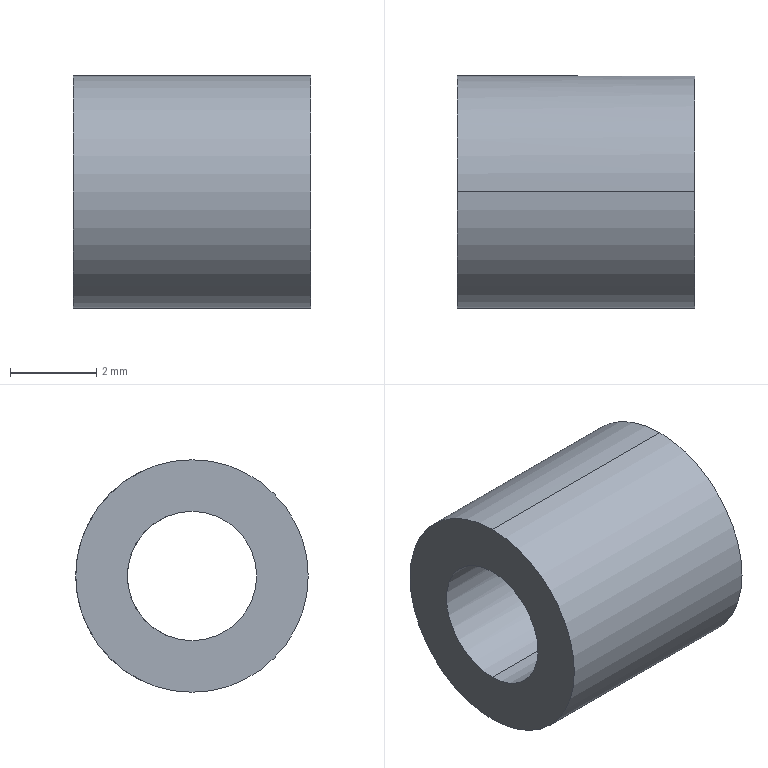Part | STEP file | RJ-HMS7-01_X2_58F34F5394A391D_1 | 1 solid | 6 faces | box 5.5 x 5.39 x 5.39 mm | volume 86.619 mm3 | cylinder 4 | plane 2 | commonest cylinder face diameters 3 x2 5.39 x2
STEP:
#1=CARTESIAN_POINT('',(0.,0.,0.));
#2=DIRECTION('',(0.,0.,1.));
#3=DIRECTION('',(1.,0.,0.));
#4=AXIS2_PLACEMENT_3D('',#1,#2,#3);
#5=CARTESIAN_POINT('',(762.8,4073.828,1374.941));
#6=VERTEX_POINT('',#5);
#7=CARTESIAN_POINT('',(762.8,4076.523,1372.246));
#8=VERTEX_POINT('',#7);
#9=CARTESIAN_POINT('',(762.8,4073.828,1372.246));
#10=DIRECTION('',(-1.,0.,0.));
#11=DIRECTION('',(0.,0.,1.));
#12=AXIS2_PLACEMENT_3D('',#9,#10,#11);
#13=CIRCLE('',#12,2.695);
#14=CARTESIAN_POINT('',(762.8,4073.828,1372.246));
#15=DIRECTION('',(1.,0.,0.));
#16=DIRECTION('',(0.,0.,-1.));
#17=AXIS2_PLACEMENT_3D('',#14,#15,#16);
#18=CYLINDRICAL_SURFACE('',#17,2.695);
#19=CARTESIAN_POINT('',(3.142,0.));
#20=DIRECTION('',(-1.,0.));
#21=VECTOR('',#20,1.);
#22=LINE('',#19,#21);
#23=(GEOMETRIC_REPRESENTATION_CONTEXT(2)PARAMETRIC_REPRESENTATION_CONTEXT()REPRESENTATION_CONTEXT('',''));
#24=DEFINITIONAL_REPRESENTATION('',(#22),#23);
#25=PCURVE('',#18,#24);
#26=CARTESIAN_POINT('',(762.8,4073.828,1372.246));
#27=DIRECTION('',(-1.,0.,0.));
#28=DIRECTION('',(0.,0.,1.));
#29=AXIS2_PLACEMENT_3D('',#26,#27,#28);
#30=PLANE('',#29);
#31=CARTESIAN_POINT('',(0.,0.));
#32=DIRECTION('',(1.,0.));
#33=AXIS2_PLACEMENT_2D('',#31,#32);
#34=CIRCLE('',#33,2.695);
#35=(GEOMETRIC_REPRESENTATION_CONTEXT(2)PARAMETRIC_REPRESENTATION_CONTEXT()REPRESENTATION_CONTEXT('',''));
#36=DEFINITIONAL_REPRESENTATION('',(#34),#35);
#37=PCURVE('',#30,#36);
#38=SURFACE_CURVE('',#13,(#25,#37),.PCURVE_S1.);
#39=EDGE_CURVE('',#6,#8,#38,.T.);
#40=ORIENTED_EDGE('',*,*,#39,.F.);
#41=CARTESIAN_POINT('',(768.3,4073.828,1374.941));
#42=VERTEX_POINT('',#41);
#43=CARTESIAN_POINT('',(762.8,4073.828,1374.941));
#44=DIRECTION('',(1.,0.,0.));
#45=VECTOR('',#44,1.);
#46=LINE('',#43,#45);
#47=CARTESIAN_POINT('',(3.142,0.));
#48=DIRECTION('',(0.,1.));
#49=VECTOR('',#48,1.);
#50=LINE('',#47,#49);
#51=(GEOMETRIC_REPRESENTATION_CONTEXT(2)PARAMETRIC_REPRESENTATION_CONTEXT()REPRESENTATION_CONTEXT('',''));
#52=DEFINITIONAL_REPRESENTATION('',(#50),#51);
#53=PCURVE('',#18,#52);
#54=CARTESIAN_POINT('',(762.8,4073.828,1372.246));
#55=DIRECTION('',(1.,0.,0.));
#56=DIRECTION('',(0.,0.,-1.));
#57=AXIS2_PLACEMENT_3D('',#54,#55,#56);
#58=CYLINDRICAL_SURFACE('',#57,2.695);
#59=CARTESIAN_POINT('',(3.142,0.));
#60=DIRECTION('',(0.,1.));
#61=VECTOR('',#60,1.);
#62=LINE('',#59,#61);
#63=(GEOMETRIC_REPRESENTATION_CONTEXT(2)PARAMETRIC_REPRESENTATION_CONTEXT()REPRESENTATION_CONTEXT('',''));
#64=DEFINITIONAL_REPRESENTATION('',(#62),#63);
#65=PCURVE('',#58,#64);
#66=SURFACE_CURVE('',#46,(#53,#65),.PCURVE_S1.);
#67=EDGE_CURVE('',#6,#42,#66,.T.);
#68=ORIENTED_EDGE('',*,*,#67,.T.);
#69=CARTESIAN_POINT('',(768.3,4073.828,1369.551));
#70=VERTEX_POINT('',#69);
#71=CARTESIAN_POINT('',(768.3,4073.828,1372.246));
#72=DIRECTION('',(1.,0.,0.));
#73=DIRECTION('',(0.,0.,-1.));
#74=AXIS2_PLACEMENT_3D('',#71,#72,#73);
#75=CIRCLE('',#74,2.695);
#76=CARTESIAN_POINT('',(0.,5.5));
#77=DIRECTION('',(1.,0.));
#78=VECTOR('',#77,1.);
#79=LINE('',#76,#78);
#80=(GEOMETRIC_REPRESENTATION_CONTEXT(2)PARAMETRIC_REPRESENTATION_CONTEXT()REPRESENTATION_CONTEXT('',''));
#81=DEFINITIONAL_REPRESENTATION('',(#79),#80);
#82=PCURVE('',#18,#81);
#83=CARTESIAN_POINT('',(768.3,4073.828,1372.246));
#84=DIRECTION('',(-1.,0.,0.));
#85=DIRECTION('',(0.,0.,1.));
#86=AXIS2_PLACEMENT_3D('',#83,#84,#85);
#87=PLANE('',#86);
#88=CARTESIAN_POINT('',(-2.695,0.));
#89=CARTESIAN_POINT('',(-2.695,4.668));
#90=CARTESIAN_POINT('',(1.347,2.334));
#91=CARTESIAN_POINT('',(5.39,0.));
#92=CARTESIAN_POINT('',(1.347,-2.334));
#93=CARTESIAN_POINT('',(-2.695,-4.668));
#94=CARTESIAN_POINT('',(-2.695,0.));
#95=(BOUNDED_CURVE()B_SPLINE_CURVE(2,(#88,#89,#90,#91,#92,#93,#94),.UNSPECIFIED.,.T.,.F.)B_SPLINE_CURVE_WITH_KNOTS((1,2,2,2,2,1),(-2.094,0.,2.094,4.189,6.283,8.378),.UNSPECIFIED.)CURVE()GEOMETRIC_REPRESENTATION_ITEM()RATIONAL_B_SPLINE_CURVE((1.,0.5,1.,0.5,1.,0.5,1.))REPRESENTATION_ITEM(''));
#96=(GEOMETRIC_REPRESENTATION_CONTEXT(2)PARAMETRIC_REPRESENTATION_CONTEXT()REPRESENTATION_CONTEXT('',''));
#97=DEFINITIONAL_REPRESENTATION('',(#95),#96);
#98=PCURVE('',#87,#97);
#99=SURFACE_CURVE('',#75,(#82,#98),.PCURVE_S1.);
#100=EDGE_CURVE('',#70,#42,#99,.T.);
#101=ORIENTED_EDGE('',*,*,#100,.F.);
#102=CARTESIAN_POINT('',(762.8,4073.828,1369.551));
#103=VERTEX_POINT('',#102);
#104=CARTESIAN_POINT('',(762.8,4073.828,1369.551));
#105=DIRECTION('',(1.,0.,0.));
#106=VECTOR('',#105,1.);
#107=LINE('',#104,#106);
#108=CARTESIAN_POINT('',(0.,0.));
#109=DIRECTION('',(0.,1.));
#110=VECTOR('',#109,1.);
#111=LINE('',#108,#110);
#112=(GEOMETRIC_REPRESENTATION_CONTEXT(2)PARAMETRIC_REPRESENTATION_CONTEXT()REPRESENTATION_CONTEXT('',''));
#113=DEFINITIONAL_REPRESENTATION('',(#111),#112);
#114=PCURVE('',#18,#113);
#115=CARTESIAN_POINT('',(6.283,0.));
#116=DIRECTION('',(0.,1.));
#117=VECTOR('',#116,1.);
#118=LINE('',#115,#117);
#119=(GEOMETRIC_REPRESENTATION_CONTEXT(2)PARAMETRIC_REPRESENTATION_CONTEXT()REPRESENTATION_CONTEXT('',''));
#120=DEFINITIONAL_REPRESENTATION('',(#118),#119);
#121=PCURVE('',#58,#120);
#122=SURFACE_CURVE('',#107,(#114,#121),.PCURVE_S1.);
#123=EDGE_CURVE('',#103,#70,#122,.T.);
#124=ORIENTED_EDGE('',*,*,#123,.F.);
#125=CARTESIAN_POINT('',(762.8,4073.828,1372.246));
#126=DIRECTION('',(-1.,0.,0.));
#127=DIRECTION('',(0.,1.,0.));
#128=AXIS2_PLACEMENT_3D('',#125,#126,#127);
#129=CIRCLE('',#128,2.695);
#130=CARTESIAN_POINT('',(1.571,0.));
#131=DIRECTION('',(-1.,0.));
#132=VECTOR('',#131,1.);
#133=LINE('',#130,#132);
#134=(GEOMETRIC_REPRESENTATION_CONTEXT(2)PARAMETRIC_REPRESENTATION_CONTEXT()REPRESENTATION_CONTEXT('',''));
#135=DEFINITIONAL_REPRESENTATION('',(#133),#134);
#136=PCURVE('',#18,#135);
#137=CARTESIAN_POINT('',(0.,0.));
#138=DIRECTION('',(0.,1.));
#139=AXIS2_PLACEMENT_2D('',#137,#138);
#140=CIRCLE('',#139,2.695);
#141=(GEOMETRIC_REPRESENTATION_CONTEXT(2)PARAMETRIC_REPRESENTATION_CONTEXT()REPRESENTATION_CONTEXT('',''));
#142=DEFINITIONAL_REPRESENTATION('',(#140),#141);
#143=PCURVE('',#30,#142);
#144=SURFACE_CURVE('',#129,(#136,#143),.PCURVE_S1.);
#145=EDGE_CURVE('',#8,#103,#144,.T.);
#146=ORIENTED_EDGE('',*,*,#145,.F.);
#147=EDGE_LOOP('',(#40,#68,#101,#124,#146));
#148=FACE_BOUND('',#147,.T.);
#149=ADVANCED_FACE('',(#148),#18,.T.);
#150=CARTESIAN_POINT('',(762.8,4071.133,1372.246));
#151=VERTEX_POINT('',#150);
#152=CARTESIAN_POINT('',(762.8,4073.828,1372.246));
#153=DIRECTION('',(-1.,0.,0.));
#154=DIRECTION('',(0.,-1.,0.));
#155=AXIS2_PLACEMENT_3D('',#152,#153,#154);
#156=CIRCLE('',#155,2.695);
#157=CARTESIAN_POINT('',(0.,0.));
#158=DIRECTION('',(0.,-1.));
#159=AXIS2_PLACEMENT_2D('',#157,#158);
#160=CIRCLE('',#159,2.695);
#161=(GEOMETRIC_REPRESENTATION_CONTEXT(2)PARAMETRIC_REPRESENTATION_CONTEXT()REPRESENTATION_CONTEXT('',''));
#162=DEFINITIONAL_REPRESENTATION('',(#160),#161);
#163=PCURVE('',#30,#162);
#164=CARTESIAN_POINT('',(4.712,0.));
#165=DIRECTION('',(-1.,0.));
#166=VECTOR('',#165,1.);
#167=LINE('',#164,#166);
#168=(GEOMETRIC_REPRESENTATION_CONTEXT(2)PARAMETRIC_REPRESENTATION_CONTEXT()REPRESENTATION_CONTEXT('',''));
#169=DEFINITIONAL_REPRESENTATION('',(#167),#168);
#170=PCURVE('',#58,#169);
#171=SURFACE_CURVE('',#156,(#163,#170),.PCURVE_S1.);
#172=EDGE_CURVE('',#151,#6,#171,.T.);
#173=ORIENTED_EDGE('',*,*,#172,.F.);
#174=CARTESIAN_POINT('',(762.8,4073.828,1372.246));
#175=DIRECTION('',(-1.,0.,0.));
#176=DIRECTION('',(0.,0.,-1.));
#177=AXIS2_PLACEMENT_3D('',#174,#175,#176);
#178=CIRCLE('',#177,2.695);
#179=CARTESIAN_POINT('',(0.,0.));
#180=DIRECTION('',(-1.,0.));
#181=AXIS2_PLACEMENT_2D('',#179,#180);
#182=CIRCLE('',#181,2.695);
#183=(GEOMETRIC_REPRESENTATION_CONTEXT(2)PARAMETRIC_REPRESENTATION_CONTEXT()REPRESENTATION_CONTEXT('',''));
#184=DEFINITIONAL_REPRESENTATION('',(#182),#183);
#185=PCURVE('',#30,#184);
#186=CARTESIAN_POINT('',(6.283,0.));
#187=DIRECTION('',(-1.,0.));
#188=VECTOR('',#187,1.);
#189=LINE('',#186,#188);
#190=(GEOMETRIC_REPRESENTATION_CONTEXT(2)PARAMETRIC_REPRESENTATION_CONTEXT()REPRESENTATION_CONTEXT('',''));
#191=DEFINITIONAL_REPRESENTATION('',(#189),#190);
#192=PCURVE('',#58,#191);
#193=SURFACE_CURVE('',#178,(#185,#192),.PCURVE_S1.);
#194=EDGE_CURVE('',#103,#151,#193,.T.);
#195=ORIENTED_EDGE('',*,*,#194,.F.);
#196=ORIENTED_EDGE('',*,*,#145,.F.);
#197=ORIENTED_EDGE('',*,*,#39,.F.);
#198=EDGE_LOOP('',(#173,#195,#196,#197));
#199=FACE_BOUND('',#198,.F.);
#200=CARTESIAN_POINT('',(762.8,4072.328,1372.246));
#201=VERTEX_POINT('',#200);
#202=CARTESIAN_POINT('',(762.8,4073.828,1370.746));
#203=VERTEX_POINT('',#202);
#204=CARTESIAN_POINT('',(762.8,4073.828,1372.246));
#205=DIRECTION('',(1.,0.,0.));
#206=DIRECTION('',(0.,-1.,0.));
#207=AXIS2_PLACEMENT_3D('',#204,#205,#206);
#208=CIRCLE('',#207,1.5);
#209=CARTESIAN_POINT('',(0.,-1.5));
#210=CARTESIAN_POINT('',(-2.598,-1.5));
#211=CARTESIAN_POINT('',(-1.299,0.75));
#212=CARTESIAN_POINT('',(0.,3.));
#213=CARTESIAN_POINT('',(1.299,0.75));
#214=CARTESIAN_POINT('',(2.598,-1.5));
#215=CARTESIAN_POINT('',(0.,-1.5));
#216=(BOUNDED_CURVE()B_SPLINE_CURVE(2,(#209,#210,#211,#212,#213,#214,#215),.UNSPECIFIED.,.T.,.F.)B_SPLINE_CURVE_WITH_KNOTS((1,2,2,2,2,1),(-2.094,0.,2.094,4.189,6.283,8.378),.UNSPECIFIED.)CURVE()GEOMETRIC_REPRESENTATION_ITEM()RATIONAL_B_SPLINE_CURVE((1.,0.5,1.,0.5,1.,0.5,1.))REPRESENTATION_ITEM(''));
#217=(GEOMETRIC_REPRESENTATION_CONTEXT(2)PARAMETRIC_REPRESENTATION_CONTEXT()REPRESENTATION_CONTEXT('',''));
#218=DEFINITIONAL_REPRESENTATION('',(#216),#217);
#219=PCURVE('',#30,#218);
#220=CARTESIAN_POINT('',(762.8,4073.828,1372.246));
#221=DIRECTION('',(1.,0.,0.));
#222=DIRECTION('',(0.,0.,-1.));
#223=AXIS2_PLACEMENT_3D('',#220,#221,#222);
#224=CYLINDRICAL_SURFACE('',#223,1.5);
#225=CARTESIAN_POINT('',(4.712,0.));
#226=DIRECTION('',(1.,0.));
#227=VECTOR('',#226,1.);
#228=LINE('',#225,#227);
#229=(GEOMETRIC_REPRESENTATION_CONTEXT(2)PARAMETRIC_REPRESENTATION_CONTEXT()REPRESENTATION_CONTEXT('',''));
#230=DEFINITIONAL_REPRESENTATION('',(#228),#229);
#231=PCURVE('',#224,#230);
#232=SURFACE_CURVE('',#208,(#219,#231),.PCURVE_S1.);
#233=EDGE_CURVE('',#201,#203,#232,.T.);
#234=ORIENTED_EDGE('',*,*,#233,.F.);
#235=CARTESIAN_POINT('',(762.8,4073.828,1373.746));
#236=VERTEX_POINT('',#235);
#237=CARTESIAN_POINT('',(762.8,4073.828,1372.246));
#238=DIRECTION('',(1.,0.,0.));
#239=DIRECTION('',(0.,0.,1.));
#240=AXIS2_PLACEMENT_3D('',#237,#238,#239);
#241=CIRCLE('',#240,1.5);
#242=CARTESIAN_POINT('',(1.5,0.));
#243=CARTESIAN_POINT('',(1.5,-2.598));
#244=CARTESIAN_POINT('',(-0.75,-1.299));
#245=CARTESIAN_POINT('',(-3.,0.));
#246=CARTESIAN_POINT('',(-0.75,1.299));
#247=CARTESIAN_POINT('',(1.5,2.598));
#248=CARTESIAN_POINT('',(1.5,0.));
#249=(BOUNDED_CURVE()B_SPLINE_CURVE(2,(#242,#243,#244,#245,#246,#247,#248),.UNSPECIFIED.,.T.,.F.)B_SPLINE_CURVE_WITH_KNOTS((1,2,2,2,2,1),(-2.094,0.,2.094,4.189,6.283,8.378),.UNSPECIFIED.)CURVE()GEOMETRIC_REPRESENTATION_ITEM()RATIONAL_B_SPLINE_CURVE((1.,0.5,1.,0.5,1.,0.5,1.))REPRESENTATION_ITEM(''));
#250=(GEOMETRIC_REPRESENTATION_CONTEXT(2)PARAMETRIC_REPRESENTATION_CONTEXT()REPRESENTATION_CONTEXT('',''));
#251=DEFINITIONAL_REPRESENTATION('',(#249),#250);
#252=PCURVE('',#30,#251);
#253=CARTESIAN_POINT('',(3.142,0.));
#254=DIRECTION('',(1.,0.));
#255=VECTOR('',#254,1.);
#256=LINE('',#253,#255);
#257=(GEOMETRIC_REPRESENTATION_CONTEXT(2)PARAMETRIC_REPRESENTATION_CONTEXT()REPRESENTATION_CONTEXT('',''));
#258=DEFINITIONAL_REPRESENTATION('',(#256),#257);
#259=PCURVE('',#224,#258);
#260=SURFACE_CURVE('',#241,(#252,#259),.PCURVE_S1.);
#261=EDGE_CURVE('',#236,#201,#260,.T.);
#262=ORIENTED_EDGE('',*,*,#261,.F.);
#263=CARTESIAN_POINT('',(762.8,4073.828,1372.246));
#264=DIRECTION('',(1.,0.,0.));
#265=DIRECTION('',(0.,0.,-1.));
#266=AXIS2_PLACEMENT_3D('',#263,#264,#265);
#267=CIRCLE('',#266,1.5);
#268=CARTESIAN_POINT('',(-1.5,0.));
#269=CARTESIAN_POINT('',(-1.5,2.598));
#270=CARTESIAN_POINT('',(0.75,1.299));
#271=CARTESIAN_POINT('',(3.,0.));
#272=CARTESIAN_POINT('',(0.75,-1.299));
#273=CARTESIAN_POINT('',(-1.5,-2.598));
#274=CARTESIAN_POINT('',(-1.5,0.));
#275=(BOUNDED_CURVE()B_SPLINE_CURVE(2,(#268,#269,#270,#271,#272,#273,#274),.UNSPECIFIED.,.T.,.F.)B_SPLINE_CURVE_WITH_KNOTS((1,2,2,2,2,1),(-2.094,0.,2.094,4.189,6.283,8.378),.UNSPECIFIED.)CURVE()GEOMETRIC_REPRESENTATION_ITEM()RATIONAL_B_SPLINE_CURVE((1.,0.5,1.,0.5,1.,0.5,1.))REPRESENTATION_ITEM(''));
#276=(GEOMETRIC_REPRESENTATION_CONTEXT(2)PARAMETRIC_REPRESENTATION_CONTEXT()REPRESENTATION_CONTEXT('',''));
#277=DEFINITIONAL_REPRESENTATION('',(#275),#276);
#278=PCURVE('',#30,#277);
#279=CARTESIAN_POINT('',(762.8,4073.828,1372.246));
#280=DIRECTION('',(1.,0.,0.));
#281=DIRECTION('',(0.,0.,-1.));
#282=AXIS2_PLACEMENT_3D('',#279,#280,#281);
#283=CYLINDRICAL_SURFACE('',#282,1.5);
#284=CARTESIAN_POINT('',(0.,0.));
#285=DIRECTION('',(1.,0.));
#286=VECTOR('',#285,1.);
#287=LINE('',#284,#286);
#288=(GEOMETRIC_REPRESENTATION_CONTEXT(2)PARAMETRIC_REPRESENTATION_CONTEXT()REPRESENTATION_CONTEXT('',''));
#289=DEFINITIONAL_REPRESENTATION('',(#287),#288);
#290=PCURVE('',#283,#289);
#291=SURFACE_CURVE('',#267,(#278,#290),.PCURVE_S1.);
#292=EDGE_CURVE('',#203,#236,#291,.T.);
#293=ORIENTED_EDGE('',*,*,#292,.F.);
#294=EDGE_LOOP('',(#234,#262,#293));
#295=FACE_BOUND('',#294,.F.);
#296=ADVANCED_FACE('',(#199,#295),#30,.T.);
#297=ORIENTED_EDGE('',*,*,#123,.T.);
#298=CARTESIAN_POINT('',(768.3,4071.133,1372.246));
#299=VERTEX_POINT('',#298);
#300=CARTESIAN_POINT('',(768.3,4073.828,1372.246));
#301=DIRECTION('',(1.,0.,0.));
#302=DIRECTION('',(0.,-1.,0.));
#303=AXIS2_PLACEMENT_3D('',#300,#301,#302);
#304=CIRCLE('',#303,2.695);
#305=CARTESIAN_POINT('',(4.712,5.5));
#306=DIRECTION('',(1.,0.));
#307=VECTOR('',#306,1.);
#308=LINE('',#305,#307);
#309=(GEOMETRIC_REPRESENTATION_CONTEXT(2)PARAMETRIC_REPRESENTATION_CONTEXT()REPRESENTATION_CONTEXT('',''));
#310=DEFINITIONAL_REPRESENTATION('',(#308),#309);
#311=PCURVE('',#58,#310);
#312=CARTESIAN_POINT('',(0.,-2.695));
#313=CARTESIAN_POINT('',(-4.668,-2.695));
#314=CARTESIAN_POINT('',(-2.334,1.347));
#315=CARTESIAN_POINT('',(0.,5.39));
#316=CARTESIAN_POINT('',(2.334,1.347));
#317=CARTESIAN_POINT('',(4.668,-2.695));
#318=CARTESIAN_POINT('',(0.,-2.695));
#319=(BOUNDED_CURVE()B_SPLINE_CURVE(2,(#312,#313,#314,#315,#316,#317,#318),.UNSPECIFIED.,.T.,.F.)B_SPLINE_CURVE_WITH_KNOTS((1,2,2,2,2,1),(-2.094,0.,2.094,4.189,6.283,8.378),.UNSPECIFIED.)CURVE()GEOMETRIC_REPRESENTATION_ITEM()RATIONAL_B_SPLINE_CURVE((1.,0.5,1.,0.5,1.,0.5,1.))REPRESENTATION_ITEM(''));
#320=(GEOMETRIC_REPRESENTATION_CONTEXT(2)PARAMETRIC_REPRESENTATION_CONTEXT()REPRESENTATION_CONTEXT('',''));
#321=DEFINITIONAL_REPRESENTATION('',(#319),#320);
#322=PCURVE('',#87,#321);
#323=SURFACE_CURVE('',#304,(#311,#322),.PCURVE_S1.);
#324=EDGE_CURVE('',#299,#70,#323,.T.);
#325=ORIENTED_EDGE('',*,*,#324,.F.);
#326=CARTESIAN_POINT('',(768.3,4073.828,1372.246));
#327=DIRECTION('',(1.,0.,0.));
#328=DIRECTION('',(0.,0.,1.));
#329=AXIS2_PLACEMENT_3D('',#326,#327,#328);
#330=CIRCLE('',#329,2.695);
#331=CARTESIAN_POINT('',(3.142,5.5));
#332=DIRECTION('',(1.,0.));
#333=VECTOR('',#332,1.);
#334=LINE('',#331,#333);
#335=(GEOMETRIC_REPRESENTATION_CONTEXT(2)PARAMETRIC_REPRESENTATION_CONTEXT()REPRESENTATION_CONTEXT('',''));
#336=DEFINITIONAL_REPRESENTATION('',(#334),#335);
#337=PCURVE('',#58,#336);
#338=CARTESIAN_POINT('',(2.695,0.));
#339=CARTESIAN_POINT('',(2.695,-4.668));
#340=CARTESIAN_POINT('',(-1.347,-2.334));
#341=CARTESIAN_POINT('',(-5.39,0.));
#342=CARTESIAN_POINT('',(-1.347,2.334));
#343=CARTESIAN_POINT('',(2.695,4.668));
#344=CARTESIAN_POINT('',(2.695,0.));
#345=(BOUNDED_CURVE()B_SPLINE_CURVE(2,(#338,#339,#340,#341,#342,#343,#344),.UNSPECIFIED.,.T.,.F.)B_SPLINE_CURVE_WITH_KNOTS((1,2,2,2,2,1),(-2.094,0.,2.094,4.189,6.283,8.378),.UNSPECIFIED.)CURVE()GEOMETRIC_REPRESENTATION_ITEM()RATIONAL_B_SPLINE_CURVE((1.,0.5,1.,0.5,1.,0.5,1.))REPRESENTATION_ITEM(''));
#346=(GEOMETRIC_REPRESENTATION_CONTEXT(2)PARAMETRIC_REPRESENTATION_CONTEXT()REPRESENTATION_CONTEXT('',''));
#347=DEFINITIONAL_REPRESENTATION('',(#345),#346);
#348=PCURVE('',#87,#347);
#349=SURFACE_CURVE('',#330,(#337,#348),.PCURVE_S1.);
#350=EDGE_CURVE('',#42,#299,#349,.T.);
#351=ORIENTED_EDGE('',*,*,#350,.F.);
#352=ORIENTED_EDGE('',*,*,#67,.F.);
#353=ORIENTED_EDGE('',*,*,#172,.F.);
#354=ORIENTED_EDGE('',*,*,#194,.F.);
#355=EDGE_LOOP('',(#297,#325,#351,#352,#353,#354));
#356=FACE_BOUND('',#355,.T.);
#357=ADVANCED_FACE('',(#356),#58,.T.);
#358=ORIENTED_EDGE('',*,*,#324,.F.);
#359=ORIENTED_EDGE('',*,*,#350,.F.);
#360=ORIENTED_EDGE('',*,*,#100,.F.);
#361=EDGE_LOOP('',(#358,#359,#360));
#362=FACE_BOUND('',#361,.F.);
#363=CARTESIAN_POINT('',(768.3,4072.328,1372.246));
#364=VERTEX_POINT('',#363);
#365=CARTESIAN_POINT('',(768.3,4073.828,1373.746));
#366=VERTEX_POINT('',#365);
#367=CARTESIAN_POINT('',(768.3,4073.828,1372.246));
#368=DIRECTION('',(-1.,0.,0.));
#369=DIRECTION('',(0.,-1.,0.));
#370=AXIS2_PLACEMENT_3D('',#367,#368,#369);
#371=CIRCLE('',#370,1.5);
#372=CARTESIAN_POINT('',(0.,0.));
#373=DIRECTION('',(0.,-1.));
#374=AXIS2_PLACEMENT_2D('',#372,#373);
#375=CIRCLE('',#374,1.5);
#376=(GEOMETRIC_REPRESENTATION_CONTEXT(2)PARAMETRIC_REPRESENTATION_CONTEXT()REPRESENTATION_CONTEXT('',''));
#377=DEFINITIONAL_REPRESENTATION('',(#375),#376);
#378=PCURVE('',#87,#377);
#379=CARTESIAN_POINT('',(4.712,5.5));
#380=DIRECTION('',(-1.,0.));
#381=VECTOR('',#380,1.);
#382=LINE('',#379,#381);
#383=(GEOMETRIC_REPRESENTATION_CONTEXT(2)PARAMETRIC_REPRESENTATION_CONTEXT()REPRESENTATION_CONTEXT('',''));
#384=DEFINITIONAL_REPRESENTATION('',(#382),#383);
#385=PCURVE('',#224,#384);
#386=SURFACE_CURVE('',#371,(#378,#385),.PCURVE_S1.);
#387=EDGE_CURVE('',#364,#366,#386,.T.);
#388=ORIENTED_EDGE('',*,*,#387,.F.);
#389=CARTESIAN_POINT('',(768.3,4073.828,1370.746));
#390=VERTEX_POINT('',#389);
#391=CARTESIAN_POINT('',(768.3,4073.828,1372.246));
#392=DIRECTION('',(-1.,0.,0.));
#393=DIRECTION('',(0.,0.,-1.));
#394=AXIS2_PLACEMENT_3D('',#391,#392,#393);
#395=CIRCLE('',#394,1.5);
#396=CARTESIAN_POINT('',(0.,0.));
#397=DIRECTION('',(-1.,0.));
#398=AXIS2_PLACEMENT_2D('',#396,#397);
#399=CIRCLE('',#398,1.5);
#400=(GEOMETRIC_REPRESENTATION_CONTEXT(2)PARAMETRIC_REPRESENTATION_CONTEXT()REPRESENTATION_CONTEXT('',''));
#401=DEFINITIONAL_REPRESENTATION('',(#399),#400);
#402=PCURVE('',#87,#401);
#403=CARTESIAN_POINT('',(6.283,5.5));
#404=DIRECTION('',(-1.,0.));
#405=VECTOR('',#404,1.);
#406=LINE('',#403,#405);
#407=(GEOMETRIC_REPRESENTATION_CONTEXT(2)PARAMETRIC_REPRESENTATION_CONTEXT()REPRESENTATION_CONTEXT('',''));
#408=DEFINITIONAL_REPRESENTATION('',(#406),#407);
#409=PCURVE('',#224,#408);
#410=SURFACE_CURVE('',#395,(#402,#409),.PCURVE_S1.);
#411=EDGE_CURVE('',#390,#364,#410,.T.);
#412=ORIENTED_EDGE('',*,*,#411,.F.);
#413=CARTESIAN_POINT('',(768.3,4075.328,1372.246));
#414=VERTEX_POINT('',#413);
#415=CARTESIAN_POINT('',(768.3,4073.828,1372.246));
#416=DIRECTION('',(-1.,0.,0.));
#417=DIRECTION('',(0.,1.,0.));
#418=AXIS2_PLACEMENT_3D('',#415,#416,#417);
#419=CIRCLE('',#418,1.5);
#420=CARTESIAN_POINT('',(0.,0.));
#421=DIRECTION('',(0.,1.));
#422=AXIS2_PLACEMENT_2D('',#420,#421);
#423=CIRCLE('',#422,1.5);
#424=(GEOMETRIC_REPRESENTATION_CONTEXT(2)PARAMETRIC_REPRESENTATION_CONTEXT()REPRESENTATION_CONTEXT('',''));
#425=DEFINITIONAL_REPRESENTATION('',(#423),#424);
#426=PCURVE('',#87,#425);
#427=CARTESIAN_POINT('',(1.571,5.5));
#428=DIRECTION('',(-1.,0.));
#429=VECTOR('',#428,1.);
#430=LINE('',#427,#429);
#431=(GEOMETRIC_REPRESENTATION_CONTEXT(2)PARAMETRIC_REPRESENTATION_CONTEXT()REPRESENTATION_CONTEXT('',''));
#432=DEFINITIONAL_REPRESENTATION('',(#430),#431);
#433=PCURVE('',#283,#432);
#434=SURFACE_CURVE('',#419,(#426,#433),.PCURVE_S1.);
#435=EDGE_CURVE('',#414,#390,#434,.T.);
#436=ORIENTED_EDGE('',*,*,#435,.F.);
#437=CARTESIAN_POINT('',(768.3,4073.828,1372.246));
#438=DIRECTION('',(-1.,0.,0.));
#439=DIRECTION('',(0.,0.,1.));
#440=AXIS2_PLACEMENT_3D('',#437,#438,#439);
#441=CIRCLE('',#440,1.5);
#442=CARTESIAN_POINT('',(0.,0.));
#443=DIRECTION('',(1.,0.));
#444=AXIS2_PLACEMENT_2D('',#442,#443);
#445=CIRCLE('',#444,1.5);
#446=(GEOMETRIC_REPRESENTATION_CONTEXT(2)PARAMETRIC_REPRESENTATION_CONTEXT()REPRESENTATION_CONTEXT('',''));
#447=DEFINITIONAL_REPRESENTATION('',(#445),#446);
#448=PCURVE('',#87,#447);
#449=CARTESIAN_POINT('',(3.142,5.5));
#450=DIRECTION('',(-1.,0.));
#451=VECTOR('',#450,1.);
#452=LINE('',#449,#451);
#453=(GEOMETRIC_REPRESENTATION_CONTEXT(2)PARAMETRIC_REPRESENTATION_CONTEXT()REPRESENTATION_CONTEXT('',''));
#454=DEFINITIONAL_REPRESENTATION('',(#452),#453);
#455=PCURVE('',#283,#454);
#456=SURFACE_CURVE('',#441,(#448,#455),.PCURVE_S1.);
#457=EDGE_CURVE('',#366,#414,#456,.T.);
#458=ORIENTED_EDGE('',*,*,#457,.F.);
#459=EDGE_LOOP('',(#388,#412,#436,#458));
#460=FACE_BOUND('',#459,.F.);
#461=ADVANCED_FACE('',(#362,#460),#87,.F.);
#462=ORIENTED_EDGE('',*,*,#261,.T.);
#463=ORIENTED_EDGE('',*,*,#233,.T.);
#464=CARTESIAN_POINT('',(762.8,4073.828,1370.746));
#465=DIRECTION('',(1.,0.,0.));
#466=VECTOR('',#465,1.);
#467=LINE('',#464,#466);
#468=CARTESIAN_POINT('',(6.283,0.));
#469=DIRECTION('',(0.,1.));
#470=VECTOR('',#469,1.);
#471=LINE('',#468,#470);
#472=(GEOMETRIC_REPRESENTATION_CONTEXT(2)PARAMETRIC_REPRESENTATION_CONTEXT()REPRESENTATION_CONTEXT('',''));
#473=DEFINITIONAL_REPRESENTATION('',(#471),#472);
#474=PCURVE('',#224,#473);
#475=CARTESIAN_POINT('',(0.,0.));
#476=DIRECTION('',(0.,1.));
#477=VECTOR('',#476,1.);
#478=LINE('',#475,#477);
#479=(GEOMETRIC_REPRESENTATION_CONTEXT(2)PARAMETRIC_REPRESENTATION_CONTEXT()REPRESENTATION_CONTEXT('',''));
#480=DEFINITIONAL_REPRESENTATION('',(#478),#479);
#481=PCURVE('',#283,#480);
#482=SURFACE_CURVE('',#467,(#474,#481),.PCURVE_S1.);
#483=EDGE_CURVE('',#203,#390,#482,.T.);
#484=ORIENTED_EDGE('',*,*,#483,.T.);
#485=ORIENTED_EDGE('',*,*,#411,.T.);
#486=ORIENTED_EDGE('',*,*,#387,.T.);
#487=CARTESIAN_POINT('',(762.8,4073.828,1373.746));
#488=DIRECTION('',(1.,0.,0.));
#489=VECTOR('',#488,1.);
#490=LINE('',#487,#489);
#491=CARTESIAN_POINT('',(3.142,0.));
#492=DIRECTION('',(0.,1.));
#493=VECTOR('',#492,1.);
#494=LINE('',#491,#493);
#495=(GEOMETRIC_REPRESENTATION_CONTEXT(2)PARAMETRIC_REPRESENTATION_CONTEXT()REPRESENTATION_CONTEXT('',''));
#496=DEFINITIONAL_REPRESENTATION('',(#494),#495);
#497=PCURVE('',#224,#496);
#498=CARTESIAN_POINT('',(3.142,0.));
#499=DIRECTION('',(0.,1.));
#500=VECTOR('',#499,1.);
#501=LINE('',#498,#500);
#502=(GEOMETRIC_REPRESENTATION_CONTEXT(2)PARAMETRIC_REPRESENTATION_CONTEXT()REPRESENTATION_CONTEXT('',''));
#503=DEFINITIONAL_REPRESENTATION('',(#501),#502);
#504=PCURVE('',#283,#503);
#505=SURFACE_CURVE('',#490,(#497,#504),.PCURVE_S1.);
#506=EDGE_CURVE('',#236,#366,#505,.T.);
#507=ORIENTED_EDGE('',*,*,#506,.F.);
#508=EDGE_LOOP('',(#462,#463,#484,#485,#486,#507));
#509=FACE_BOUND('',#508,.F.);
#510=ADVANCED_FACE('',(#509),#224,.F.);
#511=ORIENTED_EDGE('',*,*,#292,.T.);
#512=ORIENTED_EDGE('',*,*,#506,.T.);
#513=ORIENTED_EDGE('',*,*,#457,.T.);
#514=ORIENTED_EDGE('',*,*,#435,.T.);
#515=ORIENTED_EDGE('',*,*,#483,.F.);
#516=EDGE_LOOP('',(#511,#512,#513,#514,#515));
#517=FACE_BOUND('',#516,.F.);
#518=ADVANCED_FACE('',(#517),#283,.F.);
#519=CLOSED_SHELL('',(#149,#296,#357,#461,#510,#518));
#520=MANIFOLD_SOLID_BREP('',#519);
#521=(LENGTH_UNIT()NAMED_UNIT(*)SI_UNIT(.MILLI.,.METRE.));
#522=UNCERTAINTY_MEASURE_WITH_UNIT(LENGTH_MEASURE(0.0000001),#521,'','');
#523=(NAMED_UNIT(*)PLANE_ANGLE_UNIT()SI_UNIT($,.RADIAN.));
#524=(NAMED_UNIT(*)SI_UNIT($,.STERADIAN.)SOLID_ANGLE_UNIT());
#525=(GEOMETRIC_REPRESENTATION_CONTEXT(3)GLOBAL_UNCERTAINTY_ASSIGNED_CONTEXT((#522))GLOBAL_UNIT_ASSIGNED_CONTEXT((#521,#523,#524))REPRESENTATION_CONTEXT('',''));
#526=ADVANCED_BREP_SHAPE_REPRESENTATION('',(#4,#520),#525);